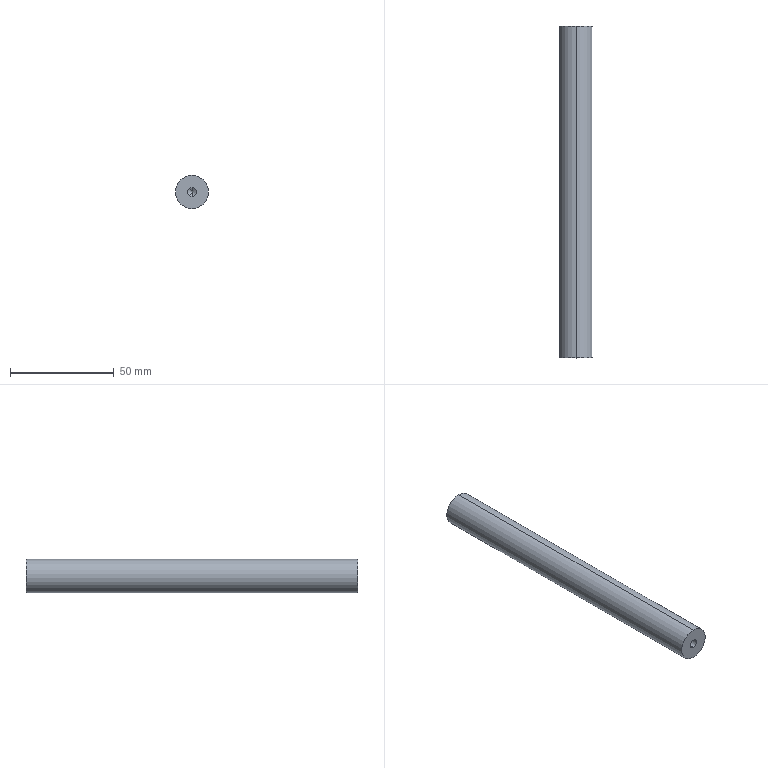Part | STEP file | PSFJW16-160-M5-N5 | 1 solid | 12 faces | box 16 x 160 x 16 mm | volume 31815 mm3 | cylinder 6 | cone 4 | plane 2 | commonest cylinder face diameters 4.2 x4 16 x2
STEP:
#1=CARTESIAN_POINT('',(0.,0.,0.));
#2=DIRECTION('',(0.,0.,1.));
#3=DIRECTION('',(1.,0.,0.));
#4=AXIS2_PLACEMENT_3D('',#1,#2,#3);
#5=CARTESIAN_POINT('',(0.,12.4,-2.1));
#6=VERTEX_POINT('',#5);
#7=CARTESIAN_POINT('',(0.,0.,-2.1));
#8=VERTEX_POINT('',#7);
#9=CARTESIAN_POINT('',(0.,0.,-2.1));
#10=DIRECTION('',(0.,-1.,0.));
#11=VECTOR('',#10,1.);
#12=LINE('',#9,#11);
#13=CARTESIAN_POINT('',(0.,0.,0.));
#14=DIRECTION('',(0.,-1.,0.));
#15=DIRECTION('',(0.,0.,-1.));
#16=AXIS2_PLACEMENT_3D('',#13,#14,#15);
#17=CYLINDRICAL_SURFACE('',#16,2.1);
#18=CARTESIAN_POINT('',(6.283,0.));
#19=DIRECTION('',(0.,1.));
#20=VECTOR('',#19,1.);
#21=LINE('',#18,#20);
#22=(GEOMETRIC_REPRESENTATION_CONTEXT(2)PARAMETRIC_REPRESENTATION_CONTEXT()REPRESENTATION_CONTEXT('',''));
#23=DEFINITIONAL_REPRESENTATION('',(#21),#22);
#24=PCURVE('',#17,#23);
#25=CARTESIAN_POINT('',(0.,0.,0.));
#26=DIRECTION('',(0.,-1.,0.));
#27=DIRECTION('',(0.,0.,-1.));
#28=AXIS2_PLACEMENT_3D('',#25,#26,#27);
#29=CYLINDRICAL_SURFACE('',#28,2.1);
#30=CARTESIAN_POINT('',(0.,0.));
#31=DIRECTION('',(0.,1.));
#32=VECTOR('',#31,1.);
#33=LINE('',#30,#32);
#34=(GEOMETRIC_REPRESENTATION_CONTEXT(2)PARAMETRIC_REPRESENTATION_CONTEXT()REPRESENTATION_CONTEXT('',''));
#35=DEFINITIONAL_REPRESENTATION('',(#33),#34);
#36=PCURVE('',#29,#35);
#37=SURFACE_CURVE('',#12,(#24,#36),.PCURVE_S1.);
#38=EDGE_CURVE('',#6,#8,#37,.T.);
#39=ORIENTED_EDGE('',*,*,#38,.T.);
#40=CARTESIAN_POINT('',(0.,0.,2.1));
#41=VERTEX_POINT('',#40);
#42=CARTESIAN_POINT('',(0.,0.,0.));
#43=DIRECTION('',(0.,-1.,0.));
#44=DIRECTION('',(0.,0.,-1.));
#45=AXIS2_PLACEMENT_3D('',#42,#43,#44);
#46=CIRCLE('',#45,2.1);
#47=CARTESIAN_POINT('',(0.,0.));
#48=DIRECTION('',(1.,0.));
#49=VECTOR('',#48,1.);
#50=LINE('',#47,#49);
#51=(GEOMETRIC_REPRESENTATION_CONTEXT(2)PARAMETRIC_REPRESENTATION_CONTEXT()REPRESENTATION_CONTEXT('',''));
#52=DEFINITIONAL_REPRESENTATION('',(#50),#51);
#53=PCURVE('',#17,#52);
#54=CARTESIAN_POINT('',(0.,0.,0.));
#55=DIRECTION('',(0.,1.,0.));
#56=DIRECTION('',(0.,0.,1.));
#57=AXIS2_PLACEMENT_3D('',#54,#55,#56);
#58=PLANE('',#57);
#59=CARTESIAN_POINT('',(-2.1,0.));
#60=CARTESIAN_POINT('',(-2.1,3.637));
#61=CARTESIAN_POINT('',(1.05,1.819));
#62=CARTESIAN_POINT('',(4.2,0.));
#63=CARTESIAN_POINT('',(1.05,-1.819));
#64=CARTESIAN_POINT('',(-2.1,-3.637));
#65=CARTESIAN_POINT('',(-2.1,0.));
#66=(BOUNDED_CURVE()B_SPLINE_CURVE(2,(#59,#60,#61,#62,#63,#64,#65),.UNSPECIFIED.,.T.,.F.)B_SPLINE_CURVE_WITH_KNOTS((1,2,2,2,2,1),(-2.094,0.,2.094,4.189,6.283,8.378),.UNSPECIFIED.)CURVE()GEOMETRIC_REPRESENTATION_ITEM()RATIONAL_B_SPLINE_CURVE((1.,0.5,1.,0.5,1.,0.5,1.))REPRESENTATION_ITEM(''));
#67=(GEOMETRIC_REPRESENTATION_CONTEXT(2)PARAMETRIC_REPRESENTATION_CONTEXT()REPRESENTATION_CONTEXT('',''));
#68=DEFINITIONAL_REPRESENTATION('',(#66),#67);
#69=PCURVE('',#58,#68);
#70=SURFACE_CURVE('',#46,(#53,#69),.PCURVE_S1.);
#71=EDGE_CURVE('',#41,#8,#70,.T.);
#72=ORIENTED_EDGE('',*,*,#71,.F.);
#73=CARTESIAN_POINT('',(0.,12.4,2.1));
#74=VERTEX_POINT('',#73);
#75=CARTESIAN_POINT('',(0.,0.,2.1));
#76=DIRECTION('',(0.,-1.,0.));
#77=VECTOR('',#76,1.);
#78=LINE('',#75,#77);
#79=CARTESIAN_POINT('',(3.142,0.));
#80=DIRECTION('',(0.,1.));
#81=VECTOR('',#80,1.);
#82=LINE('',#79,#81);
#83=(GEOMETRIC_REPRESENTATION_CONTEXT(2)PARAMETRIC_REPRESENTATION_CONTEXT()REPRESENTATION_CONTEXT('',''));
#84=DEFINITIONAL_REPRESENTATION('',(#82),#83);
#85=PCURVE('',#17,#84);
#86=CARTESIAN_POINT('',(3.142,0.));
#87=DIRECTION('',(0.,1.));
#88=VECTOR('',#87,1.);
#89=LINE('',#86,#88);
#90=(GEOMETRIC_REPRESENTATION_CONTEXT(2)PARAMETRIC_REPRESENTATION_CONTEXT()REPRESENTATION_CONTEXT('',''));
#91=DEFINITIONAL_REPRESENTATION('',(#89),#90);
#92=PCURVE('',#29,#91);
#93=SURFACE_CURVE('',#78,(#85,#92),.PCURVE_S1.);
#94=EDGE_CURVE('',#74,#41,#93,.T.);
#95=ORIENTED_EDGE('',*,*,#94,.F.);
#96=CARTESIAN_POINT('',(0.,12.4,0.));
#97=DIRECTION('',(0.,-1.,0.));
#98=DIRECTION('',(0.,0.,-1.));
#99=AXIS2_PLACEMENT_3D('',#96,#97,#98);
#100=CIRCLE('',#99,2.1);
#101=CARTESIAN_POINT('',(0.,-12.4));
#102=DIRECTION('',(1.,0.));
#103=VECTOR('',#102,1.);
#104=LINE('',#101,#103);
#105=(GEOMETRIC_REPRESENTATION_CONTEXT(2)PARAMETRIC_REPRESENTATION_CONTEXT()REPRESENTATION_CONTEXT('',''));
#106=DEFINITIONAL_REPRESENTATION('',(#104),#105);
#107=PCURVE('',#17,#106);
#108=CARTESIAN_POINT('',(0.,12.4,0.));
#109=DIRECTION('',(0.,-1.,0.));
#110=DIRECTION('',(0.,0.,-1.));
#111=AXIS2_PLACEMENT_3D('',#108,#109,#110);
#112=CONICAL_SURFACE('',#111,2.1,1.03);
#113=CARTESIAN_POINT('',(0.,0.));
#114=DIRECTION('',(1.,0.));
#115=VECTOR('',#114,1.);
#116=LINE('',#113,#115);
#117=(GEOMETRIC_REPRESENTATION_CONTEXT(2)PARAMETRIC_REPRESENTATION_CONTEXT()REPRESENTATION_CONTEXT('',''));
#118=DEFINITIONAL_REPRESENTATION('',(#116),#117);
#119=PCURVE('',#112,#118);
#120=SURFACE_CURVE('',#100,(#107,#119),.PCURVE_S1.);
#121=EDGE_CURVE('',#74,#6,#120,.T.);
#122=ORIENTED_EDGE('',*,*,#121,.T.);
#123=EDGE_LOOP('',(#39,#72,#95,#122));
#124=FACE_BOUND('',#123,.F.);
#125=ADVANCED_FACE('',(#124),#17,.F.);
#126=ORIENTED_EDGE('',*,*,#121,.F.);
#127=CARTESIAN_POINT('',(0.,13.662,0.));
#128=VERTEX_POINT('',#127);
#129=CARTESIAN_POINT('',(0.,12.4,2.1));
#130=DIRECTION('',(0.,-0.515,0.8572));
#131=VECTOR('',#130,1.);
#132=LINE('',#129,#131);
#133=CARTESIAN_POINT('',(3.142,0.));
#134=DIRECTION('',(0.,1.));
#135=VECTOR('',#134,1.);
#136=LINE('',#133,#135);
#137=(GEOMETRIC_REPRESENTATION_CONTEXT(2)PARAMETRIC_REPRESENTATION_CONTEXT()REPRESENTATION_CONTEXT('',''));
#138=DEFINITIONAL_REPRESENTATION('',(#136),#137);
#139=PCURVE('',#112,#138);
#140=CARTESIAN_POINT('',(0.,12.4,0.));
#141=DIRECTION('',(0.,-1.,0.));
#142=DIRECTION('',(0.,0.,-1.));
#143=AXIS2_PLACEMENT_3D('',#140,#141,#142);
#144=CONICAL_SURFACE('',#143,2.1,1.03);
#145=CARTESIAN_POINT('',(3.142,0.));
#146=DIRECTION('',(0.,1.));
#147=VECTOR('',#146,1.);
#148=LINE('',#145,#147);
#149=(GEOMETRIC_REPRESENTATION_CONTEXT(2)PARAMETRIC_REPRESENTATION_CONTEXT()REPRESENTATION_CONTEXT('',''));
#150=DEFINITIONAL_REPRESENTATION('',(#148),#149);
#151=PCURVE('',#144,#150);
#152=SURFACE_CURVE('',#132,(#139,#151),.PCURVE_S1.);
#153=EDGE_CURVE('',#128,#74,#152,.T.);
#154=ORIENTED_EDGE('',*,*,#153,.F.);
#155=CARTESIAN_POINT('',(0.,12.4,-2.1));
#156=DIRECTION('',(0.,-0.515,-0.8572));
#157=VECTOR('',#156,1.);
#158=LINE('',#155,#157);
#159=CARTESIAN_POINT('',(6.283,0.));
#160=DIRECTION('',(0.,1.));
#161=VECTOR('',#160,1.);
#162=LINE('',#159,#161);
#163=(GEOMETRIC_REPRESENTATION_CONTEXT(2)PARAMETRIC_REPRESENTATION_CONTEXT()REPRESENTATION_CONTEXT('',''));
#164=DEFINITIONAL_REPRESENTATION('',(#162),#163);
#165=PCURVE('',#112,#164);
#166=CARTESIAN_POINT('',(0.,0.));
#167=DIRECTION('',(0.,1.));
#168=VECTOR('',#167,1.);
#169=LINE('',#166,#168);
#170=(GEOMETRIC_REPRESENTATION_CONTEXT(2)PARAMETRIC_REPRESENTATION_CONTEXT()REPRESENTATION_CONTEXT('',''));
#171=DEFINITIONAL_REPRESENTATION('',(#169),#170);
#172=PCURVE('',#144,#171);
#173=SURFACE_CURVE('',#158,(#165,#172),.PCURVE_S1.);
#174=EDGE_CURVE('',#128,#6,#173,.T.);
#175=ORIENTED_EDGE('',*,*,#174,.T.);
#176=EDGE_LOOP('',(#126,#154,#175));
#177=FACE_BOUND('',#176,.F.);
#178=ADVANCED_FACE('',(#177),#112,.F.);
#179=CARTESIAN_POINT('',(0.,147.6,2.1));
#180=VERTEX_POINT('',#179);
#181=CARTESIAN_POINT('',(0.,160.,2.1));
#182=VERTEX_POINT('',#181);
#183=CARTESIAN_POINT('',(0.,160.,2.1));
#184=DIRECTION('',(0.,1.,0.));
#185=VECTOR('',#184,1.);
#186=LINE('',#183,#185);
#187=CARTESIAN_POINT('',(0.,160.,0.));
#188=DIRECTION('',(0.,1.,0.));
#189=DIRECTION('',(0.,0.,1.));
#190=AXIS2_PLACEMENT_3D('',#187,#188,#189);
#191=CYLINDRICAL_SURFACE('',#190,2.1);
#192=CARTESIAN_POINT('',(6.283,0.));
#193=DIRECTION('',(0.,1.));
#194=VECTOR('',#193,1.);
#195=LINE('',#192,#194);
#196=(GEOMETRIC_REPRESENTATION_CONTEXT(2)PARAMETRIC_REPRESENTATION_CONTEXT()REPRESENTATION_CONTEXT('',''));
#197=DEFINITIONAL_REPRESENTATION('',(#195),#196);
#198=PCURVE('',#191,#197);
#199=CARTESIAN_POINT('',(0.,160.,0.));
#200=DIRECTION('',(0.,1.,0.));
#201=DIRECTION('',(0.,0.,1.));
#202=AXIS2_PLACEMENT_3D('',#199,#200,#201);
#203=CYLINDRICAL_SURFACE('',#202,2.1);
#204=CARTESIAN_POINT('',(0.,0.));
#205=DIRECTION('',(0.,1.));
#206=VECTOR('',#205,1.);
#207=LINE('',#204,#206);
#208=(GEOMETRIC_REPRESENTATION_CONTEXT(2)PARAMETRIC_REPRESENTATION_CONTEXT()REPRESENTATION_CONTEXT('',''));
#209=DEFINITIONAL_REPRESENTATION('',(#207),#208);
#210=PCURVE('',#203,#209);
#211=SURFACE_CURVE('',#186,(#198,#210),.PCURVE_S1.);
#212=EDGE_CURVE('',#180,#182,#211,.T.);
#213=ORIENTED_EDGE('',*,*,#212,.T.);
#214=CARTESIAN_POINT('',(0.,160.,-2.1));
#215=VERTEX_POINT('',#214);
#216=CARTESIAN_POINT('',(0.,160.,0.));
#217=DIRECTION('',(0.,1.,0.));
#218=DIRECTION('',(0.,0.,1.));
#219=AXIS2_PLACEMENT_3D('',#216,#217,#218);
#220=CIRCLE('',#219,2.1);
#221=CARTESIAN_POINT('',(0.,0.));
#222=DIRECTION('',(1.,0.));
#223=VECTOR('',#222,1.);
#224=LINE('',#221,#223);
#225=(GEOMETRIC_REPRESENTATION_CONTEXT(2)PARAMETRIC_REPRESENTATION_CONTEXT()REPRESENTATION_CONTEXT('',''));
#226=DEFINITIONAL_REPRESENTATION('',(#224),#225);
#227=PCURVE('',#191,#226);
#228=CARTESIAN_POINT('',(0.,160.,0.));
#229=DIRECTION('',(0.,1.,0.));
#230=DIRECTION('',(0.,0.,1.));
#231=AXIS2_PLACEMENT_3D('',#228,#229,#230);
#232=PLANE('',#231);
#233=CARTESIAN_POINT('',(0.,0.));
#234=DIRECTION('',(1.,0.));
#235=AXIS2_PLACEMENT_2D('',#233,#234);
#236=CIRCLE('',#235,2.1);
#237=(GEOMETRIC_REPRESENTATION_CONTEXT(2)PARAMETRIC_REPRESENTATION_CONTEXT()REPRESENTATION_CONTEXT('',''));
#238=DEFINITIONAL_REPRESENTATION('',(#236),#237);
#239=PCURVE('',#232,#238);
#240=SURFACE_CURVE('',#220,(#227,#239),.PCURVE_S1.);
#241=EDGE_CURVE('',#215,#182,#240,.T.);
#242=ORIENTED_EDGE('',*,*,#241,.F.);
#243=CARTESIAN_POINT('',(0.,147.6,-2.1));
#244=VERTEX_POINT('',#243);
#245=CARTESIAN_POINT('',(0.,160.,-2.1));
#246=DIRECTION('',(0.,1.,0.));
#247=VECTOR('',#246,1.);
#248=LINE('',#245,#247);
#249=CARTESIAN_POINT('',(3.142,0.));
#250=DIRECTION('',(0.,1.));
#251=VECTOR('',#250,1.);
#252=LINE('',#249,#251);
#253=(GEOMETRIC_REPRESENTATION_CONTEXT(2)PARAMETRIC_REPRESENTATION_CONTEXT()REPRESENTATION_CONTEXT('',''));
#254=DEFINITIONAL_REPRESENTATION('',(#252),#253);
#255=PCURVE('',#191,#254);
#256=CARTESIAN_POINT('',(3.142,0.));
#257=DIRECTION('',(0.,1.));
#258=VECTOR('',#257,1.);
#259=LINE('',#256,#258);
#260=(GEOMETRIC_REPRESENTATION_CONTEXT(2)PARAMETRIC_REPRESENTATION_CONTEXT()REPRESENTATION_CONTEXT('',''));
#261=DEFINITIONAL_REPRESENTATION('',(#259),#260);
#262=PCURVE('',#203,#261);
#263=SURFACE_CURVE('',#248,(#255,#262),.PCURVE_S1.);
#264=EDGE_CURVE('',#244,#215,#263,.T.);
#265=ORIENTED_EDGE('',*,*,#264,.F.);
#266=CARTESIAN_POINT('',(0.,147.6,0.));
#267=DIRECTION('',(0.,1.,0.));
#268=DIRECTION('',(0.,0.,1.));
#269=AXIS2_PLACEMENT_3D('',#266,#267,#268);
#270=CIRCLE('',#269,2.1);
#271=CARTESIAN_POINT('',(0.,-12.4));
#272=DIRECTION('',(1.,0.));
#273=VECTOR('',#272,1.);
#274=LINE('',#271,#273);
#275=(GEOMETRIC_REPRESENTATION_CONTEXT(2)PARAMETRIC_REPRESENTATION_CONTEXT()REPRESENTATION_CONTEXT('',''));
#276=DEFINITIONAL_REPRESENTATION('',(#274),#275);
#277=PCURVE('',#191,#276);
#278=CARTESIAN_POINT('',(0.,147.6,0.));
#279=DIRECTION('',(0.,1.,0.));
#280=DIRECTION('',(0.,0.,1.));
#281=AXIS2_PLACEMENT_3D('',#278,#279,#280);
#282=CONICAL_SURFACE('',#281,2.1,1.03);
#283=CARTESIAN_POINT('',(0.,0.));
#284=DIRECTION('',(1.,0.));
#285=VECTOR('',#284,1.);
#286=LINE('',#283,#285);
#287=(GEOMETRIC_REPRESENTATION_CONTEXT(2)PARAMETRIC_REPRESENTATION_CONTEXT()REPRESENTATION_CONTEXT('',''));
#288=DEFINITIONAL_REPRESENTATION('',(#286),#287);
#289=PCURVE('',#282,#288);
#290=SURFACE_CURVE('',#270,(#277,#289),.PCURVE_S1.);
#291=EDGE_CURVE('',#244,#180,#290,.T.);
#292=ORIENTED_EDGE('',*,*,#291,.T.);
#293=EDGE_LOOP('',(#213,#242,#265,#292));
#294=FACE_BOUND('',#293,.F.);
#295=ADVANCED_FACE('',(#294),#191,.F.);
#296=ORIENTED_EDGE('',*,*,#291,.F.);
#297=CARTESIAN_POINT('',(0.,146.338,0.));
#298=VERTEX_POINT('',#297);
#299=CARTESIAN_POINT('',(0.,147.6,-2.1));
#300=DIRECTION('',(0.,0.515,-0.8572));
#301=VECTOR('',#300,1.);
#302=LINE('',#299,#301);
#303=CARTESIAN_POINT('',(3.142,-1.262));
#304=CARTESIAN_POINT('',(3.142,-1.243));
#305=CARTESIAN_POINT('',(3.142,-1.204));
#306=CARTESIAN_POINT('',(3.142,-1.147));
#307=CARTESIAN_POINT('',(3.142,-1.09));
#308=CARTESIAN_POINT('',(3.142,-1.032));
#309=CARTESIAN_POINT('',(3.142,-0.975));
#310=CARTESIAN_POINT('',(3.142,-0.9177));
#311=CARTESIAN_POINT('',(3.142,-0.8603));
#312=CARTESIAN_POINT('',(3.142,-0.803));
#313=CARTESIAN_POINT('',(3.142,-0.7456));
#314=CARTESIAN_POINT('',(3.142,-0.6883));
#315=CARTESIAN_POINT('',(3.142,-0.6309));
#316=CARTESIAN_POINT('',(3.142,-0.5735));
#317=CARTESIAN_POINT('',(3.142,-0.5162));
#318=CARTESIAN_POINT('',(3.142,-0.4588));
#319=CARTESIAN_POINT('',(3.142,-0.4015));
#320=CARTESIAN_POINT('',(3.142,-0.3441));
#321=CARTESIAN_POINT('',(3.142,-0.2868));
#322=CARTESIAN_POINT('',(3.142,-0.2294));
#323=CARTESIAN_POINT('',(3.142,-0.1721));
#324=CARTESIAN_POINT('',(3.142,-0.1147));
#325=CARTESIAN_POINT('',(3.142,-0.05735));
#326=CARTESIAN_POINT('',(3.142,-0.01912));
#327=CARTESIAN_POINT('',(3.142,0.));
#328=B_SPLINE_CURVE_WITH_KNOTS('',3,(#303,#304,#305,#306,#307,#308,#309,#310,#311,#312,#313,#314,#315,#316,#317,#318,#319,#320,#321,#322,#323,#324,#325,#326,#327),.UNSPECIFIED.,.F.,.F.,(4,1,1,1,1,1,1,1,1,1,1,1,1,1,1,1,1,1,1,1,1,1,4),(-2.45,-2.339,-2.227,-2.116,-2.004,-1.893,-1.782,-1.67,-1.559,-1.448,-1.336,-1.225,-1.114,-1.002,-0.8909,-0.7795,-0.6682,-0.5568,-0.4454,-0.3341,-0.2227,-0.1114,0.),.UNSPECIFIED.);
#329=(GEOMETRIC_REPRESENTATION_CONTEXT(2)PARAMETRIC_REPRESENTATION_CONTEXT()REPRESENTATION_CONTEXT('',''));
#330=DEFINITIONAL_REPRESENTATION('',(#328),#329);
#331=PCURVE('',#282,#330);
#332=CARTESIAN_POINT('',(0.,147.6,0.));
#333=DIRECTION('',(0.,1.,0.));
#334=DIRECTION('',(0.,0.,1.));
#335=AXIS2_PLACEMENT_3D('',#332,#333,#334);
#336=CONICAL_SURFACE('',#335,2.1,1.03);
#337=CARTESIAN_POINT('',(3.142,-1.262));
#338=CARTESIAN_POINT('',(3.142,-1.243));
#339=CARTESIAN_POINT('',(3.142,-1.204));
#340=CARTESIAN_POINT('',(3.142,-1.147));
#341=CARTESIAN_POINT('',(3.142,-1.09));
#342=CARTESIAN_POINT('',(3.142,-1.032));
#343=CARTESIAN_POINT('',(3.142,-0.975));
#344=CARTESIAN_POINT('',(3.142,-0.9177));
#345=CARTESIAN_POINT('',(3.142,-0.8603));
#346=CARTESIAN_POINT('',(3.142,-0.803));
#347=CARTESIAN_POINT('',(3.142,-0.7456));
#348=CARTESIAN_POINT('',(3.142,-0.6883));
#349=CARTESIAN_POINT('',(3.142,-0.6309));
#350=CARTESIAN_POINT('',(3.142,-0.5735));
#351=CARTESIAN_POINT('',(3.142,-0.5162));
#352=CARTESIAN_POINT('',(3.142,-0.4588));
#353=CARTESIAN_POINT('',(3.142,-0.4015));
#354=CARTESIAN_POINT('',(3.142,-0.3441));
#355=CARTESIAN_POINT('',(3.142,-0.2868));
#356=CARTESIAN_POINT('',(3.142,-0.2294));
#357=CARTESIAN_POINT('',(3.142,-0.1721));
#358=CARTESIAN_POINT('',(3.142,-0.1147));
#359=CARTESIAN_POINT('',(3.142,-0.05735));
#360=CARTESIAN_POINT('',(3.142,-0.01912));
#361=CARTESIAN_POINT('',(3.142,0.));
#362=B_SPLINE_CURVE_WITH_KNOTS('',3,(#337,#338,#339,#340,#341,#342,#343,#344,#345,#346,#347,#348,#349,#350,#351,#352,#353,#354,#355,#356,#357,#358,#359,#360,#361),.UNSPECIFIED.,.F.,.F.,(4,1,1,1,1,1,1,1,1,1,1,1,1,1,1,1,1,1,1,1,1,1,4),(-2.45,-2.339,-2.227,-2.116,-2.004,-1.893,-1.782,-1.67,-1.559,-1.448,-1.336,-1.225,-1.114,-1.002,-0.8909,-0.7795,-0.6682,-0.5568,-0.4454,-0.3341,-0.2227,-0.1114,0.),.UNSPECIFIED.);
#363=(GEOMETRIC_REPRESENTATION_CONTEXT(2)PARAMETRIC_REPRESENTATION_CONTEXT()REPRESENTATION_CONTEXT('',''));
#364=DEFINITIONAL_REPRESENTATION('',(#362),#363);
#365=PCURVE('',#336,#364);
#366=SURFACE_CURVE('',#302,(#331,#365),.PCURVE_S1.);
#367=EDGE_CURVE('',#298,#244,#366,.T.);
#368=ORIENTED_EDGE('',*,*,#367,.F.);
#369=CARTESIAN_POINT('',(0.,147.6,2.1));
#370=DIRECTION('',(0.,0.515,0.8572));
#371=VECTOR('',#370,1.);
#372=LINE('',#369,#371);
#373=CARTESIAN_POINT('',(6.283,-1.262));
#374=CARTESIAN_POINT('',(6.283,-1.243));
#375=CARTESIAN_POINT('',(6.283,-1.204));
#376=CARTESIAN_POINT('',(6.283,-1.147));
#377=CARTESIAN_POINT('',(6.283,-1.09));
#378=CARTESIAN_POINT('',(6.283,-1.032));
#379=CARTESIAN_POINT('',(6.283,-0.975));
#380=CARTESIAN_POINT('',(6.283,-0.9177));
#381=CARTESIAN_POINT('',(6.283,-0.8603));
#382=CARTESIAN_POINT('',(6.283,-0.803));
#383=CARTESIAN_POINT('',(6.283,-0.7456));
#384=CARTESIAN_POINT('',(6.283,-0.6883));
#385=CARTESIAN_POINT('',(6.283,-0.6309));
#386=CARTESIAN_POINT('',(6.283,-0.5735));
#387=CARTESIAN_POINT('',(6.283,-0.5162));
#388=CARTESIAN_POINT('',(6.283,-0.4588));
#389=CARTESIAN_POINT('',(6.283,-0.4015));
#390=CARTESIAN_POINT('',(6.283,-0.3441));
#391=CARTESIAN_POINT('',(6.283,-0.2868));
#392=CARTESIAN_POINT('',(6.283,-0.2294));
#393=CARTESIAN_POINT('',(6.283,-0.1721));
#394=CARTESIAN_POINT('',(6.283,-0.1147));
#395=CARTESIAN_POINT('',(6.283,-0.05735));
#396=CARTESIAN_POINT('',(6.283,-0.01912));
#397=CARTESIAN_POINT('',(6.283,0.));
#398=B_SPLINE_CURVE_WITH_KNOTS('',3,(#373,#374,#375,#376,#377,#378,#379,#380,#381,#382,#383,#384,#385,#386,#387,#388,#389,#390,#391,#392,#393,#394,#395,#396,#397),.UNSPECIFIED.,.F.,.F.,(4,1,1,1,1,1,1,1,1,1,1,1,1,1,1,1,1,1,1,1,1,1,4),(-2.45,-2.339,-2.227,-2.116,-2.004,-1.893,-1.782,-1.67,-1.559,-1.448,-1.336,-1.225,-1.114,-1.002,-0.8909,-0.7795,-0.6682,-0.5568,-0.4454,-0.3341,-0.2227,-0.1114,0.),.UNSPECIFIED.);
#399=(GEOMETRIC_REPRESENTATION_CONTEXT(2)PARAMETRIC_REPRESENTATION_CONTEXT()REPRESENTATION_CONTEXT('',''));
#400=DEFINITIONAL_REPRESENTATION('',(#398),#399);
#401=PCURVE('',#282,#400);
#402=CARTESIAN_POINT('',(0.,-1.262));
#403=CARTESIAN_POINT('',(0.,-1.243));
#404=CARTESIAN_POINT('',(0.,-1.204));
#405=CARTESIAN_POINT('',(0.,-1.147));
#406=CARTESIAN_POINT('',(0.,-1.09));
#407=CARTESIAN_POINT('',(0.,-1.032));
#408=CARTESIAN_POINT('',(0.,-0.975));
#409=CARTESIAN_POINT('',(0.,-0.9177));
#410=CARTESIAN_POINT('',(0.,-0.8603));
#411=CARTESIAN_POINT('',(0.,-0.803));
#412=CARTESIAN_POINT('',(0.,-0.7456));
#413=CARTESIAN_POINT('',(0.,-0.6883));
#414=CARTESIAN_POINT('',(0.,-0.6309));
#415=CARTESIAN_POINT('',(0.,-0.5735));
#416=CARTESIAN_POINT('',(0.,-0.5162));
#417=CARTESIAN_POINT('',(0.,-0.4588));
#418=CARTESIAN_POINT('',(0.,-0.4015));
#419=CARTESIAN_POINT('',(0.,-0.3441));
#420=CARTESIAN_POINT('',(0.,-0.2868));
#421=CARTESIAN_POINT('',(0.,-0.2294));
#422=CARTESIAN_POINT('',(0.,-0.1721));
#423=CARTESIAN_POINT('',(0.,-0.1147));
#424=CARTESIAN_POINT('',(0.,-0.05735));
#425=CARTESIAN_POINT('',(0.,-0.01912));
#426=CARTESIAN_POINT('',(0.,0.));
#427=B_SPLINE_CURVE_WITH_KNOTS('',3,(#402,#403,#404,#405,#406,#407,#408,#409,#410,#411,#412,#413,#414,#415,#416,#417,#418,#419,#420,#421,#422,#423,#424,#425,#426),.UNSPECIFIED.,.F.,.F.,(4,1,1,1,1,1,1,1,1,1,1,1,1,1,1,1,1,1,1,1,1,1,4),(-2.45,-2.339,-2.227,-2.116,-2.004,-1.893,-1.782,-1.67,-1.559,-1.448,-1.336,-1.225,-1.114,-1.002,-0.8909,-0.7795,-0.6682,-0.5568,-0.4454,-0.3341,-0.2227,-0.1114,0.),.UNSPECIFIED.);
#428=(GEOMETRIC_REPRESENTATION_CONTEXT(2)PARAMETRIC_REPRESENTATION_CONTEXT()REPRESENTATION_CONTEXT('',''));
#429=DEFINITIONAL_REPRESENTATION('',(#427),#428);
#430=PCURVE('',#336,#429);
#431=SURFACE_CURVE('',#372,(#401,#430),.PCURVE_S1.);
#432=EDGE_CURVE('',#298,#180,#431,.T.);
#433=ORIENTED_EDGE('',*,*,#432,.T.);
#434=EDGE_LOOP('',(#296,#368,#433));
#435=FACE_BOUND('',#434,.F.);
#436=ADVANCED_FACE('',(#435),#282,.F.);
#437=CARTESIAN_POINT('',(0.,160.,8.));
#438=VERTEX_POINT('',#437);
#439=CARTESIAN_POINT('',(0.,160.,-8.));
#440=VERTEX_POINT('',#439);
#441=CARTESIAN_POINT('',(0.,160.,0.));
#442=DIRECTION('',(0.,1.,0.));
#443=DIRECTION('',(0.,0.,1.));
#444=AXIS2_PLACEMENT_3D('',#441,#442,#443);
#445=CIRCLE('',#444,8.);
#446=CARTESIAN_POINT('',(0.,160.,0.));
#447=DIRECTION('',(0.,-1.,0.));
#448=DIRECTION('',(0.,0.,-1.));
#449=AXIS2_PLACEMENT_3D('',#446,#447,#448);
#450=CYLINDRICAL_SURFACE('',#449,8.);
#451=CARTESIAN_POINT('',(3.142,0.));
#452=DIRECTION('',(-1.,0.));
#453=VECTOR('',#452,1.);
#454=LINE('',#451,#453);
#455=(GEOMETRIC_REPRESENTATION_CONTEXT(2)PARAMETRIC_REPRESENTATION_CONTEXT()REPRESENTATION_CONTEXT('',''));
#456=DEFINITIONAL_REPRESENTATION('',(#454),#455);
#457=PCURVE('',#450,#456);
#458=CARTESIAN_POINT('',(0.,0.));
#459=DIRECTION('',(1.,0.));
#460=AXIS2_PLACEMENT_2D('',#458,#459);
#461=CIRCLE('',#460,8.);
#462=(GEOMETRIC_REPRESENTATION_CONTEXT(2)PARAMETRIC_REPRESENTATION_CONTEXT()REPRESENTATION_CONTEXT('',''));
#463=DEFINITIONAL_REPRESENTATION('',(#461),#462);
#464=PCURVE('',#232,#463);
#465=SURFACE_CURVE('',#445,(#457,#464),.PCURVE_S1.);
#466=EDGE_CURVE('',#438,#440,#465,.T.);
#467=ORIENTED_EDGE('',*,*,#466,.F.);
#468=CARTESIAN_POINT('',(0.,0.,8.));
#469=VERTEX_POINT('',#468);
#470=CARTESIAN_POINT('',(0.,160.,8.));
#471=DIRECTION('',(0.,-1.,0.));
#472=VECTOR('',#471,1.);
#473=LINE('',#470,#472);
#474=CARTESIAN_POINT('',(3.142,0.));
#475=DIRECTION('',(0.,1.));
#476=VECTOR('',#475,1.);
#477=LINE('',#474,#476);
#478=(GEOMETRIC_REPRESENTATION_CONTEXT(2)PARAMETRIC_REPRESENTATION_CONTEXT()REPRESENTATION_CONTEXT('',''));
#479=DEFINITIONAL_REPRESENTATION('',(#477),#478);
#480=PCURVE('',#450,#479);
#481=CARTESIAN_POINT('',(0.,160.,0.));
#482=DIRECTION('',(0.,-1.,0.));
#483=DIRECTION('',(0.,0.,-1.));
#484=AXIS2_PLACEMENT_3D('',#481,#482,#483);
#485=CYLINDRICAL_SURFACE('',#484,8.);
#486=CARTESIAN_POINT('',(3.142,0.));
#487=DIRECTION('',(0.,1.));
#488=VECTOR('',#487,1.);
#489=LINE('',#486,#488);
#490=(GEOMETRIC_REPRESENTATION_CONTEXT(2)PARAMETRIC_REPRESENTATION_CONTEXT()REPRESENTATION_CONTEXT('',''));
#491=DEFINITIONAL_REPRESENTATION('',(#489),#490);
#492=PCURVE('',#485,#491);
#493=SURFACE_CURVE('',#473,(#480,#492),.PCURVE_S1.);
#494=EDGE_CURVE('',#438,#469,#493,.T.);
#495=ORIENTED_EDGE('',*,*,#494,.T.);
#496=CARTESIAN_POINT('',(0.,0.,-8.));
#497=VERTEX_POINT('',#496);
#498=CARTESIAN_POINT('',(0.,0.,0.));
#499=DIRECTION('',(0.,1.,0.));
#500=DIRECTION('',(0.,0.,1.));
#501=AXIS2_PLACEMENT_3D('',#498,#499,#500);
#502=CIRCLE('',#501,8.);
#503=CARTESIAN_POINT('',(3.142,160.));
#504=DIRECTION('',(-1.,0.));
#505=VECTOR('',#504,1.);
#506=LINE('',#503,#505);
#507=(GEOMETRIC_REPRESENTATION_CONTEXT(2)PARAMETRIC_REPRESENTATION_CONTEXT()REPRESENTATION_CONTEXT('',''));
#508=DEFINITIONAL_REPRESENTATION('',(#506),#507);
#509=PCURVE('',#450,#508);
#510=CARTESIAN_POINT('',(0.,0.));
#511=DIRECTION('',(1.,0.));
#512=AXIS2_PLACEMENT_2D('',#510,#511);
#513=CIRCLE('',#512,8.);
#514=(GEOMETRIC_REPRESENTATION_CONTEXT(2)PARAMETRIC_REPRESENTATION_CONTEXT()REPRESENTATION_CONTEXT('',''));
#515=DEFINITIONAL_REPRESENTATION('',(#513),#514);
#516=PCURVE('',#58,#515);
#517=SURFACE_CURVE('',#502,(#509,#516),.PCURVE_S1.);
#518=EDGE_CURVE('',#469,#497,#517,.T.);
#519=ORIENTED_EDGE('',*,*,#518,.T.);
#520=CARTESIAN_POINT('',(0.,160.,-8.));
#521=DIRECTION('',(0.,-1.,0.));
#522=VECTOR('',#521,1.);
#523=LINE('',#520,#522);
#524=CARTESIAN_POINT('',(0.,0.));
#525=DIRECTION('',(0.,1.));
#526=VECTOR('',#525,1.);
#527=LINE('',#524,#526);
#528=(GEOMETRIC_REPRESENTATION_CONTEXT(2)PARAMETRIC_REPRESENTATION_CONTEXT()REPRESENTATION_CONTEXT('',''));
#529=DEFINITIONAL_REPRESENTATION('',(#527),#528);
#530=PCURVE('',#450,#529);
#531=CARTESIAN_POINT('',(6.283,0.));
#532=DIRECTION('',(0.,1.));
#533=VECTOR('',#532,1.);
#534=LINE('',#531,#533);
#535=(GEOMETRIC_REPRESENTATION_CONTEXT(2)PARAMETRIC_REPRESENTATION_CONTEXT()REPRESENTATION_CONTEXT('',''));
#536=DEFINITIONAL_REPRESENTATION('',(#534),#535);
#537=PCURVE('',#485,#536);
#538=SURFACE_CURVE('',#523,(#530,#537),.PCURVE_S1.);
#539=EDGE_CURVE('',#440,#497,#538,.T.);
#540=ORIENTED_EDGE('',*,*,#539,.F.);
#541=EDGE_LOOP('',(#467,#495,#519,#540));
#542=FACE_BOUND('',#541,.T.);
#543=ADVANCED_FACE('',(#542),#450,.T.);
#544=ORIENTED_EDGE('',*,*,#494,.F.);
#545=CARTESIAN_POINT('',(0.,160.,0.));
#546=DIRECTION('',(0.,1.,0.));
#547=DIRECTION('',(0.,0.,1.));
#548=AXIS2_PLACEMENT_3D('',#545,#546,#547);
#549=CIRCLE('',#548,8.);
#550=CARTESIAN_POINT('',(9.425,0.));
#551=DIRECTION('',(-1.,0.));
#552=VECTOR('',#551,1.);
#553=LINE('',#550,#552);
#554=(GEOMETRIC_REPRESENTATION_CONTEXT(2)PARAMETRIC_REPRESENTATION_CONTEXT()REPRESENTATION_CONTEXT('',''));
#555=DEFINITIONAL_REPRESENTATION('',(#553),#554);
#556=PCURVE('',#485,#555);
#557=CARTESIAN_POINT('',(0.,0.));
#558=DIRECTION('',(1.,0.));
#559=AXIS2_PLACEMENT_2D('',#557,#558);
#560=CIRCLE('',#559,8.);
#561=(GEOMETRIC_REPRESENTATION_CONTEXT(2)PARAMETRIC_REPRESENTATION_CONTEXT()REPRESENTATION_CONTEXT('',''));
#562=DEFINITIONAL_REPRESENTATION('',(#560),#561);
#563=PCURVE('',#232,#562);
#564=SURFACE_CURVE('',#549,(#556,#563),.PCURVE_S1.);
#565=EDGE_CURVE('',#440,#438,#564,.T.);
#566=ORIENTED_EDGE('',*,*,#565,.F.);
#567=ORIENTED_EDGE('',*,*,#539,.T.);
#568=CARTESIAN_POINT('',(0.,0.,0.));
#569=DIRECTION('',(0.,1.,0.));
#570=DIRECTION('',(0.,0.,1.));
#571=AXIS2_PLACEMENT_3D('',#568,#569,#570);
#572=CIRCLE('',#571,8.);
#573=CARTESIAN_POINT('',(9.425,160.));
#574=DIRECTION('',(-1.,0.));
#575=VECTOR('',#574,1.);
#576=LINE('',#573,#575);
#577=(GEOMETRIC_REPRESENTATION_CONTEXT(2)PARAMETRIC_REPRESENTATION_CONTEXT()REPRESENTATION_CONTEXT('',''));
#578=DEFINITIONAL_REPRESENTATION('',(#576),#577);
#579=PCURVE('',#485,#578);
#580=CARTESIAN_POINT('',(0.,0.));
#581=DIRECTION('',(1.,0.));
#582=AXIS2_PLACEMENT_2D('',#580,#581);
#583=CIRCLE('',#582,8.);
#584=(GEOMETRIC_REPRESENTATION_CONTEXT(2)PARAMETRIC_REPRESENTATION_CONTEXT()REPRESENTATION_CONTEXT('',''));
#585=DEFINITIONAL_REPRESENTATION('',(#583),#584);
#586=PCURVE('',#58,#585);
#587=SURFACE_CURVE('',#572,(#579,#586),.PCURVE_S1.);
#588=EDGE_CURVE('',#497,#469,#587,.T.);
#589=ORIENTED_EDGE('',*,*,#588,.T.);
#590=EDGE_LOOP('',(#544,#566,#567,#589));
#591=FACE_BOUND('',#590,.T.);
#592=ADVANCED_FACE('',(#591),#485,.T.);
#593=CARTESIAN_POINT('',(0.,160.,0.));
#594=DIRECTION('',(0.,1.,0.));
#595=DIRECTION('',(0.,0.,1.));
#596=AXIS2_PLACEMENT_3D('',#593,#594,#595);
#597=CIRCLE('',#596,2.1);
#598=CARTESIAN_POINT('',(0.,0.));
#599=DIRECTION('',(1.,0.));
#600=AXIS2_PLACEMENT_2D('',#598,#599);
#601=CIRCLE('',#600,2.1);
#602=(GEOMETRIC_REPRESENTATION_CONTEXT(2)PARAMETRIC_REPRESENTATION_CONTEXT()REPRESENTATION_CONTEXT('',''));
#603=DEFINITIONAL_REPRESENTATION('',(#601),#602);
#604=PCURVE('',#232,#603);
#605=CARTESIAN_POINT('',(0.,0.));
#606=DIRECTION('',(1.,0.));
#607=VECTOR('',#606,1.);
#608=LINE('',#605,#607);
#609=(GEOMETRIC_REPRESENTATION_CONTEXT(2)PARAMETRIC_REPRESENTATION_CONTEXT()REPRESENTATION_CONTEXT('',''));
#610=DEFINITIONAL_REPRESENTATION('',(#608),#609);
#611=PCURVE('',#203,#610);
#612=SURFACE_CURVE('',#597,(#604,#611),.PCURVE_S1.);
#613=EDGE_CURVE('',#182,#215,#612,.T.);
#614=ORIENTED_EDGE('',*,*,#613,.F.);
#615=ORIENTED_EDGE('',*,*,#241,.F.);
#616=EDGE_LOOP('',(#614,#615));
#617=FACE_BOUND('',#616,.T.);
#618=ORIENTED_EDGE('',*,*,#565,.T.);
#619=ORIENTED_EDGE('',*,*,#466,.T.);
#620=EDGE_LOOP('',(#618,#619));
#621=FACE_BOUND('',#620,.T.);
#622=ADVANCED_FACE('',(#617,#621),#232,.T.);
#623=CARTESIAN_POINT('',(0.,0.,0.));
#624=DIRECTION('',(0.,-1.,0.));
#625=DIRECTION('',(0.,0.,-1.));
#626=AXIS2_PLACEMENT_3D('',#623,#624,#625);
#627=CIRCLE('',#626,2.1);
#628=CARTESIAN_POINT('',(-2.1,0.));
#629=CARTESIAN_POINT('',(-2.1,3.637));
#630=CARTESIAN_POINT('',(1.05,1.819));
#631=CARTESIAN_POINT('',(4.2,0.));
#632=CARTESIAN_POINT('',(1.05,-1.819));
#633=CARTESIAN_POINT('',(-2.1,-3.637));
#634=CARTESIAN_POINT('',(-2.1,0.));
#635=(BOUNDED_CURVE()B_SPLINE_CURVE(2,(#628,#629,#630,#631,#632,#633,#634),.UNSPECIFIED.,.T.,.F.)B_SPLINE_CURVE_WITH_KNOTS((1,2,2,2,2,1),(-2.094,0.,2.094,4.189,6.283,8.378),.UNSPECIFIED.)CURVE()GEOMETRIC_REPRESENTATION_ITEM()RATIONAL_B_SPLINE_CURVE((1.,0.5,1.,0.5,1.,0.5,1.))REPRESENTATION_ITEM(''));
#636=(GEOMETRIC_REPRESENTATION_CONTEXT(2)PARAMETRIC_REPRESENTATION_CONTEXT()REPRESENTATION_CONTEXT('',''));
#637=DEFINITIONAL_REPRESENTATION('',(#635),#636);
#638=PCURVE('',#58,#637);
#639=CARTESIAN_POINT('',(0.,0.));
#640=DIRECTION('',(1.,0.));
#641=VECTOR('',#640,1.);
#642=LINE('',#639,#641);
#643=(GEOMETRIC_REPRESENTATION_CONTEXT(2)PARAMETRIC_REPRESENTATION_CONTEXT()REPRESENTATION_CONTEXT('',''));
#644=DEFINITIONAL_REPRESENTATION('',(#642),#643);
#645=PCURVE('',#29,#644);
#646=SURFACE_CURVE('',#627,(#638,#645),.PCURVE_S1.);
#647=EDGE_CURVE('',#8,#41,#646,.T.);
#648=ORIENTED_EDGE('',*,*,#647,.F.);
#649=ORIENTED_EDGE('',*,*,#71,.F.);
#650=EDGE_LOOP('',(#648,#649));
#651=FACE_BOUND('',#650,.T.);
#652=ORIENTED_EDGE('',*,*,#588,.F.);
#653=ORIENTED_EDGE('',*,*,#518,.F.);
#654=EDGE_LOOP('',(#652,#653));
#655=FACE_BOUND('',#654,.T.);
#656=ADVANCED_FACE('',(#651,#655),#58,.F.);
#657=CARTESIAN_POINT('',(0.,147.6,0.));
#658=DIRECTION('',(0.,1.,0.));
#659=DIRECTION('',(0.,0.,1.));
#660=AXIS2_PLACEMENT_3D('',#657,#658,#659);
#661=CIRCLE('',#660,2.1);
#662=CARTESIAN_POINT('',(0.,0.));
#663=DIRECTION('',(1.,0.));
#664=VECTOR('',#663,1.);
#665=LINE('',#662,#664);
#666=(GEOMETRIC_REPRESENTATION_CONTEXT(2)PARAMETRIC_REPRESENTATION_CONTEXT()REPRESENTATION_CONTEXT('',''));
#667=DEFINITIONAL_REPRESENTATION('',(#665),#666);
#668=PCURVE('',#336,#667);
#669=CARTESIAN_POINT('',(0.,-12.4));
#670=DIRECTION('',(1.,0.));
#671=VECTOR('',#670,1.);
#672=LINE('',#669,#671);
#673=(GEOMETRIC_REPRESENTATION_CONTEXT(2)PARAMETRIC_REPRESENTATION_CONTEXT()REPRESENTATION_CONTEXT('',''));
#674=DEFINITIONAL_REPRESENTATION('',(#672),#673);
#675=PCURVE('',#203,#674);
#676=SURFACE_CURVE('',#661,(#668,#675),.PCURVE_S1.);
#677=EDGE_CURVE('',#180,#244,#676,.T.);
#678=ORIENTED_EDGE('',*,*,#677,.F.);
#679=ORIENTED_EDGE('',*,*,#432,.F.);
#680=ORIENTED_EDGE('',*,*,#367,.T.);
#681=EDGE_LOOP('',(#678,#679,#680));
#682=FACE_BOUND('',#681,.F.);
#683=ADVANCED_FACE('',(#682),#336,.F.);
#684=ORIENTED_EDGE('',*,*,#613,.F.);
#685=ORIENTED_EDGE('',*,*,#212,.F.);
#686=ORIENTED_EDGE('',*,*,#677,.T.);
#687=ORIENTED_EDGE('',*,*,#264,.T.);
#688=EDGE_LOOP('',(#684,#685,#686,#687));
#689=FACE_BOUND('',#688,.F.);
#690=ADVANCED_FACE('',(#689),#203,.F.);
#691=CARTESIAN_POINT('',(0.,12.4,0.));
#692=DIRECTION('',(0.,-1.,0.));
#693=DIRECTION('',(0.,0.,-1.));
#694=AXIS2_PLACEMENT_3D('',#691,#692,#693);
#695=CIRCLE('',#694,2.1);
#696=CARTESIAN_POINT('',(0.,0.));
#697=DIRECTION('',(1.,0.));
#698=VECTOR('',#697,1.);
#699=LINE('',#696,#698);
#700=(GEOMETRIC_REPRESENTATION_CONTEXT(2)PARAMETRIC_REPRESENTATION_CONTEXT()REPRESENTATION_CONTEXT('',''));
#701=DEFINITIONAL_REPRESENTATION('',(#699),#700);
#702=PCURVE('',#144,#701);
#703=CARTESIAN_POINT('',(0.,-12.4));
#704=DIRECTION('',(1.,0.));
#705=VECTOR('',#704,1.);
#706=LINE('',#703,#705);
#707=(GEOMETRIC_REPRESENTATION_CONTEXT(2)PARAMETRIC_REPRESENTATION_CONTEXT()REPRESENTATION_CONTEXT('',''));
#708=DEFINITIONAL_REPRESENTATION('',(#706),#707);
#709=PCURVE('',#29,#708);
#710=SURFACE_CURVE('',#695,(#702,#709),.PCURVE_S1.);
#711=EDGE_CURVE('',#6,#74,#710,.T.);
#712=ORIENTED_EDGE('',*,*,#711,.F.);
#713=ORIENTED_EDGE('',*,*,#174,.F.);
#714=ORIENTED_EDGE('',*,*,#153,.T.);
#715=EDGE_LOOP('',(#712,#713,#714));
#716=FACE_BOUND('',#715,.F.);
#717=ADVANCED_FACE('',(#716),#144,.F.);
#718=ORIENTED_EDGE('',*,*,#647,.F.);
#719=ORIENTED_EDGE('',*,*,#38,.F.);
#720=ORIENTED_EDGE('',*,*,#711,.T.);
#721=ORIENTED_EDGE('',*,*,#94,.T.);
#722=EDGE_LOOP('',(#718,#719,#720,#721));
#723=FACE_BOUND('',#722,.F.);
#724=ADVANCED_FACE('',(#723),#29,.F.);
#725=CLOSED_SHELL('',(#125,#178,#295,#436,#543,#592,#622,#656,#683,#690,#717,#724));
#726=MANIFOLD_SOLID_BREP('',#725);
#727=(LENGTH_UNIT()NAMED_UNIT(*)SI_UNIT(.MILLI.,.METRE.));
#728=UNCERTAINTY_MEASURE_WITH_UNIT(LENGTH_MEASURE(0.0000001),#727,'','');
#729=(NAMED_UNIT(*)PLANE_ANGLE_UNIT()SI_UNIT($,.RADIAN.));
#730=(NAMED_UNIT(*)SI_UNIT($,.STERADIAN.)SOLID_ANGLE_UNIT());
#731=(GEOMETRIC_REPRESENTATION_CONTEXT(3)GLOBAL_UNCERTAINTY_ASSIGNED_CONTEXT((#728))GLOBAL_UNIT_ASSIGNED_CONTEXT((#727,#729,#730))REPRESENTATION_CONTEXT('',''));
#732=ADVANCED_BREP_SHAPE_REPRESENTATION('',(#4,#726),#731);